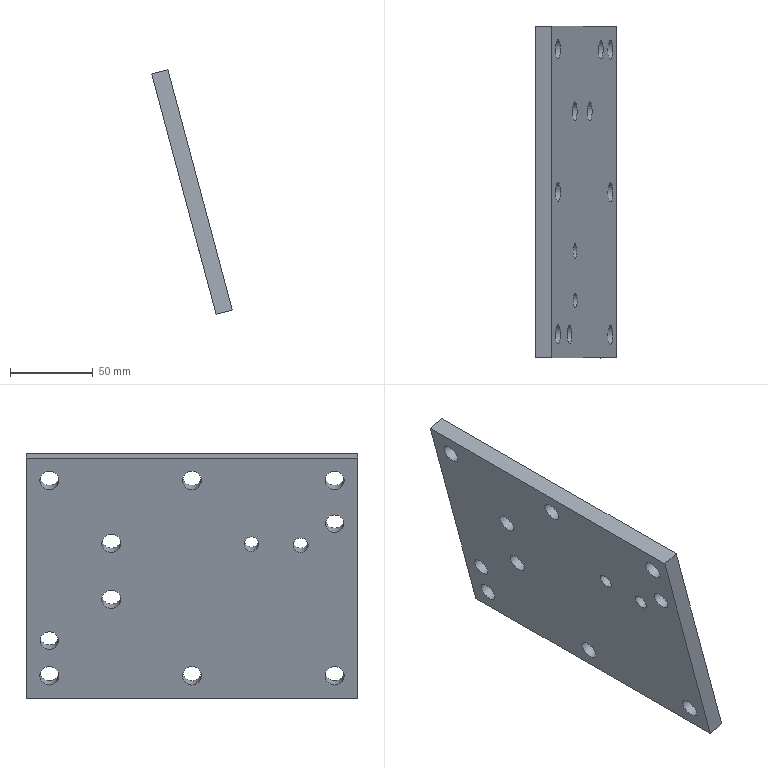Part | NX | features solid 2 | 1 solid | 18 faces | box 48.482 x 200 x 147.477 mm | volume 288505 mm3 | cylinder 12 | plane 6 | commonest cylinder face diameters 11.507 x8 9.007 x2 11 x2
STEP:
#1=CARTESIAN_POINT('',(922.389,65.937,-48.234));
#2=VERTEX_POINT('',#1);
#3=CARTESIAN_POINT('',(920.965,65.937,-42.921));
#4=DIRECTION('',(0.9659,-0.000000134,0.2588));
#5=DIRECTION('',(0.2588,0.,-0.9659));
#6=AXIS2_PLACEMENT_3D('',#3,#4,#5);
#7=CIRCLE('',#6,5.5);
#8=EDGE_CURVE('',#2,#2,#7,.F.);
#9=ORIENTED_EDGE('',*,*,#8,.F.);
#10=EDGE_LOOP('',(#9));
#11=FACE_BOUND('',#10,.T.);
#12=CARTESIAN_POINT('',(896.573,-20.063,48.114));
#13=VERTEX_POINT('',#12);
#14=CARTESIAN_POINT('',(895.084,-20.063,53.671));
#15=DIRECTION('',(0.9659,-0.000000134,0.2588));
#16=DIRECTION('',(0.2588,0.,-0.9659));
#17=AXIS2_PLACEMENT_3D('',#14,#15,#16);
#18=CIRCLE('',#17,5.753);
#19=EDGE_CURVE('',#13,#13,#18,.F.);
#20=ORIENTED_EDGE('',*,*,#19,.F.);
#21=EDGE_LOOP('',(#20));
#22=FACE_BOUND('',#21,.T.);
#23=CARTESIAN_POINT('',(928.149,-20.063,-69.729));
#24=VERTEX_POINT('',#23);
#25=CARTESIAN_POINT('',(926.659,-20.063,-64.172));
#26=DIRECTION('',(0.9659,-0.000000134,0.2588));
#27=DIRECTION('',(0.2588,0.,-0.9659));
#28=AXIS2_PLACEMENT_3D('',#25,#26,#27);
#29=CIRCLE('',#28,5.753);
#30=EDGE_CURVE('',#24,#24,#29,.T.);
#31=ORIENTED_EDGE('',*,*,#30,.T.);
#32=EDGE_LOOP('',(#31));
#33=FACE_BOUND('',#32,.T.);
#34=CARTESIAN_POINT('',(928.149,65.937,-69.729));
#35=VERTEX_POINT('',#34);
#36=CARTESIAN_POINT('',(926.659,65.937,-64.172));
#37=DIRECTION('',(0.9659,-0.000000134,0.2588));
#38=DIRECTION('',(0.2588,0.,-0.9659));
#39=AXIS2_PLACEMENT_3D('',#36,#37,#38);
#40=CIRCLE('',#39,5.753);
#41=EDGE_CURVE('',#35,#35,#40,.T.);
#42=ORIENTED_EDGE('',*,*,#41,.T.);
#43=EDGE_LOOP('',(#42));
#44=FACE_BOUND('',#43,.T.);
#45=CARTESIAN_POINT('',(891.46,-120.063,67.194));
#46=VERTEX_POINT('',#45);
#47=CARTESIAN_POINT('',(930.283,-120.063,-77.695));
#48=VERTEX_POINT('',#47);
#49=CARTESIAN_POINT('',(1072.537,-120.063,-608.595));
#50=DIRECTION('',(0.2588,0.000000499,-0.9659));
#51=VECTOR('',#50,1000.);
#52=LINE('',#49,#51);
#53=EDGE_CURVE('',#46,#48,#52,.T.);
#54=ORIENTED_EDGE('',*,*,#53,.F.);
#55=CARTESIAN_POINT('',(891.46,79.937,67.194));
#56=VERTEX_POINT('',#55);
#57=CARTESIAN_POINT('',(891.46,4.19,67.194));
#58=DIRECTION('',(0.,-1.,-0.000000517));
#59=VECTOR('',#58,1000.);
#60=LINE('',#57,#59);
#61=EDGE_CURVE('',#56,#46,#60,.T.);
#62=ORIENTED_EDGE('',*,*,#61,.F.);
#63=CARTESIAN_POINT('',(930.283,79.937,-77.695));
#64=VERTEX_POINT('',#63);
#65=CARTESIAN_POINT('',(925.107,79.937,-58.376));
#66=DIRECTION('',(-0.2588,-0.000000499,0.9659));
#67=VECTOR('',#66,1000.);
#68=LINE('',#65,#67);
#69=EDGE_CURVE('',#64,#56,#68,.T.);
#70=ORIENTED_EDGE('',*,*,#69,.F.);
#71=CARTESIAN_POINT('',(930.283,-100.063,-77.695));
#72=DIRECTION('',(0.,1.,0.000000517));
#73=VECTOR('',#72,1000.);
#74=LINE('',#71,#73);
#75=EDGE_CURVE('',#48,#64,#74,.T.);
#76=ORIENTED_EDGE('',*,*,#75,.F.);
#77=EDGE_LOOP('',(#54,#62,#70,#76));
#78=FACE_BOUND('',#77,.T.);
#79=CARTESIAN_POINT('',(915.774,28.571,-23.546));
#80=VERTEX_POINT('',#79);
#81=CARTESIAN_POINT('',(914.285,28.571,-17.988));
#82=DIRECTION('',(0.9659,-0.000000134,0.2588));
#83=DIRECTION('',(0.2588,0.,-0.9659));
#84=AXIS2_PLACEMENT_3D('',#81,#82,#83);
#85=CIRCLE('',#84,5.753);
#86=EDGE_CURVE('',#80,#80,#85,.T.);
#87=ORIENTED_EDGE('',*,*,#86,.T.);
#88=EDGE_LOOP('',(#87));
#89=FACE_BOUND('',#88,.T.);
#90=CARTESIAN_POINT('',(906.716,-85.584,10.259));
#91=VERTEX_POINT('',#90);
#92=CARTESIAN_POINT('',(905.55,-85.584,14.61));
#93=DIRECTION('',(0.9659,-0.000000134,0.2588));
#94=DIRECTION('',(0.2588,0.,-0.9659));
#95=AXIS2_PLACEMENT_3D('',#92,#93,#94);
#96=CIRCLE('',#95,4.503);
#97=EDGE_CURVE('',#91,#91,#96,.T.);
#98=ORIENTED_EDGE('',*,*,#97,.T.);
#99=EDGE_LOOP('',(#98));
#100=FACE_BOUND('',#99,.T.);
#101=CARTESIAN_POINT('',(906.538,-55.901,10.924));
#102=VERTEX_POINT('',#101);
#103=CARTESIAN_POINT('',(905.372,-55.901,15.274));
#104=DIRECTION('',(0.9659,-0.000000134,0.2588));
#105=DIRECTION('',(0.2588,0.,-0.9659));
#106=AXIS2_PLACEMENT_3D('',#103,#104,#105);
#107=CIRCLE('',#106,4.503);
#108=EDGE_CURVE('',#102,#102,#107,.T.);
#109=ORIENTED_EDGE('',*,*,#108,.T.);
#110=EDGE_LOOP('',(#109));
#111=FACE_BOUND('',#110,.T.);
#112=CARTESIAN_POINT('',(906.735,28.571,10.189));
#113=VERTEX_POINT('',#112);
#114=CARTESIAN_POINT('',(905.245,28.571,15.746));
#115=DIRECTION('',(0.9659,-0.000000134,0.2588));
#116=DIRECTION('',(0.2588,0.,-0.9659));
#117=AXIS2_PLACEMENT_3D('',#114,#115,#116);
#118=CIRCLE('',#117,5.753);
#119=EDGE_CURVE('',#113,#113,#118,.F.);
#120=ORIENTED_EDGE('',*,*,#119,.F.);
#121=EDGE_LOOP('',(#120));
#122=FACE_BOUND('',#121,.T.);
#123=CARTESIAN_POINT('',(896.573,-106.063,48.114));
#124=VERTEX_POINT('',#123);
#125=CARTESIAN_POINT('',(895.084,-106.063,53.671));
#126=DIRECTION('',(0.9659,-0.000000134,0.2588));
#127=DIRECTION('',(0.2588,0.,-0.9659));
#128=AXIS2_PLACEMENT_3D('',#125,#126,#127);
#129=CIRCLE('',#128,5.753);
#130=EDGE_CURVE('',#124,#124,#129,.T.);
#131=ORIENTED_EDGE('',*,*,#130,.T.);
#132=EDGE_LOOP('',(#131));
#133=FACE_BOUND('',#132,.T.);
#134=CARTESIAN_POINT('',(896.573,65.937,48.114));
#135=VERTEX_POINT('',#134);
#136=CARTESIAN_POINT('',(895.084,65.937,53.671));
#137=DIRECTION('',(0.9659,-0.000000134,0.2588));
#138=DIRECTION('',(0.2588,0.,-0.9659));
#139=AXIS2_PLACEMENT_3D('',#136,#137,#138);
#140=CIRCLE('',#139,5.753);
#141=EDGE_CURVE('',#135,#135,#140,.T.);
#142=ORIENTED_EDGE('',*,*,#141,.T.);
#143=EDGE_LOOP('',(#142));
#144=FACE_BOUND('',#143,.T.);
#145=CARTESIAN_POINT('',(928.149,-106.063,-69.729));
#146=VERTEX_POINT('',#145);
#147=CARTESIAN_POINT('',(926.659,-106.063,-64.172));
#148=DIRECTION('',(0.9659,-0.000000134,0.2588));
#149=DIRECTION('',(0.2588,0.,-0.9659));
#150=AXIS2_PLACEMENT_3D('',#147,#148,#149);
#151=CIRCLE('',#150,5.753);
#152=EDGE_CURVE('',#146,#146,#151,.F.);
#153=ORIENTED_EDGE('',*,*,#152,.F.);
#154=EDGE_LOOP('',(#153));
#155=FACE_BOUND('',#154,.T.);
#156=CARTESIAN_POINT('',(903.495,-106.063,22.279));
#157=VERTEX_POINT('',#156);
#158=CARTESIAN_POINT('',(902.072,-106.063,27.591));
#159=DIRECTION('',(0.9659,-0.000000134,0.2588));
#160=DIRECTION('',(0.2588,0.,-0.9659));
#161=AXIS2_PLACEMENT_3D('',#158,#159,#160);
#162=CIRCLE('',#161,5.5);
#163=EDGE_CURVE('',#157,#157,#162,.F.);
#164=ORIENTED_EDGE('',*,*,#163,.F.);
#165=EDGE_LOOP('',(#164));
#166=FACE_BOUND('',#165,.T.);
#167=CARTESIAN_POINT('',(1072.537,4.191,-608.595));
#168=DIRECTION('',(0.9659,-0.000000134,0.2588));
#169=DIRECTION('',(-0.2588,0.,0.9659));
#170=AXIS2_PLACEMENT_3D('',#167,#168,#169);
#171=PLANE('',#170);
#172=ADVANCED_FACE('',(#11,#22,#33,#44,#78,#89,#100,#111,#122,#133,#144,#155,#166),#171,.F.);
#173=CARTESIAN_POINT('',(932.048,65.937,-45.646));
#174=VERTEX_POINT('',#173);
#175=CARTESIAN_POINT('',(930.625,65.937,-40.333));
#176=DIRECTION('',(0.9659,-0.000000134,0.2588));
#177=DIRECTION('',(0.2588,0.,-0.9659));
#178=AXIS2_PLACEMENT_3D('',#175,#176,#177);
#179=CIRCLE('',#178,5.5);
#180=EDGE_CURVE('',#174,#174,#179,.F.);
#181=ORIENTED_EDGE('',*,*,#180,.T.);
#182=EDGE_LOOP('',(#181));
#183=FACE_BOUND('',#182,.T.);
#184=CARTESIAN_POINT('',(906.232,-20.063,50.702));
#185=VERTEX_POINT('',#184);
#186=CARTESIAN_POINT('',(904.743,-20.063,56.259));
#187=DIRECTION('',(0.9659,-0.000000134,0.2588));
#188=DIRECTION('',(0.2588,0.,-0.9659));
#189=AXIS2_PLACEMENT_3D('',#186,#187,#188);
#190=CIRCLE('',#189,5.753);
#191=EDGE_CURVE('',#185,#185,#190,.F.);
#192=ORIENTED_EDGE('',*,*,#191,.T.);
#193=EDGE_LOOP('',(#192));
#194=FACE_BOUND('',#193,.T.);
#195=CARTESIAN_POINT('',(937.808,-20.063,-67.141));
#196=VERTEX_POINT('',#195);
#197=CARTESIAN_POINT('',(936.319,-20.063,-61.584));
#198=DIRECTION('',(0.9659,-0.000000134,0.2588));
#199=DIRECTION('',(0.2588,0.,-0.9659));
#200=AXIS2_PLACEMENT_3D('',#197,#198,#199);
#201=CIRCLE('',#200,5.753);
#202=EDGE_CURVE('',#196,#196,#201,.T.);
#203=ORIENTED_EDGE('',*,*,#202,.F.);
#204=EDGE_LOOP('',(#203));
#205=FACE_BOUND('',#204,.T.);
#206=CARTESIAN_POINT('',(937.808,65.937,-67.141));
#207=VERTEX_POINT('',#206);
#208=CARTESIAN_POINT('',(936.319,65.937,-61.584));
#209=DIRECTION('',(0.9659,-0.000000134,0.2588));
#210=DIRECTION('',(0.2588,0.,-0.9659));
#211=AXIS2_PLACEMENT_3D('',#208,#209,#210);
#212=CIRCLE('',#211,5.753);
#213=EDGE_CURVE('',#207,#207,#212,.T.);
#214=ORIENTED_EDGE('',*,*,#213,.F.);
#215=EDGE_LOOP('',(#214));
#216=FACE_BOUND('',#215,.T.);
#217=CARTESIAN_POINT('',(901.119,-120.063,69.782));
#218=VERTEX_POINT('',#217);
#219=CARTESIAN_POINT('',(939.942,-120.063,-75.107));
#220=VERTEX_POINT('',#219);
#221=CARTESIAN_POINT('',(1082.196,-120.063,-606.006));
#222=DIRECTION('',(0.2588,0.000000499,-0.9659));
#223=VECTOR('',#222,1000.);
#224=LINE('',#221,#223);
#225=EDGE_CURVE('',#218,#220,#224,.T.);
#226=ORIENTED_EDGE('',*,*,#225,.T.);
#227=CARTESIAN_POINT('',(939.942,79.937,-75.107));
#228=VERTEX_POINT('',#227);
#229=CARTESIAN_POINT('',(939.942,-100.063,-75.107));
#230=DIRECTION('',(0.,1.,0.000000517));
#231=VECTOR('',#230,1000.);
#232=LINE('',#229,#231);
#233=EDGE_CURVE('',#220,#228,#232,.T.);
#234=ORIENTED_EDGE('',*,*,#233,.T.);
#235=CARTESIAN_POINT('',(901.119,79.937,69.782));
#236=VERTEX_POINT('',#235);
#237=CARTESIAN_POINT('',(934.766,79.937,-55.788));
#238=DIRECTION('',(-0.2588,-0.000000499,0.9659));
#239=VECTOR('',#238,1000.);
#240=LINE('',#237,#239);
#241=EDGE_CURVE('',#228,#236,#240,.T.);
#242=ORIENTED_EDGE('',*,*,#241,.T.);
#243=CARTESIAN_POINT('',(901.119,4.19,69.782));
#244=DIRECTION('',(0.,-1.,-0.000000517));
#245=VECTOR('',#244,1000.);
#246=LINE('',#243,#245);
#247=EDGE_CURVE('',#236,#218,#246,.T.);
#248=ORIENTED_EDGE('',*,*,#247,.T.);
#249=EDGE_LOOP('',(#226,#234,#242,#248));
#250=FACE_BOUND('',#249,.T.);
#251=CARTESIAN_POINT('',(925.433,28.571,-20.957));
#252=VERTEX_POINT('',#251);
#253=CARTESIAN_POINT('',(923.944,28.571,-15.4));
#254=DIRECTION('',(0.9659,-0.000000134,0.2588));
#255=DIRECTION('',(0.2588,0.,-0.9659));
#256=AXIS2_PLACEMENT_3D('',#253,#254,#255);
#257=CIRCLE('',#256,5.753);
#258=EDGE_CURVE('',#252,#252,#257,.T.);
#259=ORIENTED_EDGE('',*,*,#258,.F.);
#260=EDGE_LOOP('',(#259));
#261=FACE_BOUND('',#260,.T.);
#262=CARTESIAN_POINT('',(916.375,-85.584,12.848));
#263=VERTEX_POINT('',#262);
#264=CARTESIAN_POINT('',(915.209,-85.584,17.198));
#265=DIRECTION('',(0.9659,-0.000000134,0.2588));
#266=DIRECTION('',(0.2588,0.,-0.9659));
#267=AXIS2_PLACEMENT_3D('',#264,#265,#266);
#268=CIRCLE('',#267,4.503);
#269=EDGE_CURVE('',#263,#263,#268,.T.);
#270=ORIENTED_EDGE('',*,*,#269,.F.);
#271=EDGE_LOOP('',(#270));
#272=FACE_BOUND('',#271,.T.);
#273=CARTESIAN_POINT('',(916.197,-55.901,13.512));
#274=VERTEX_POINT('',#273);
#275=CARTESIAN_POINT('',(915.031,-55.901,17.862));
#276=DIRECTION('',(0.9659,-0.000000134,0.2588));
#277=DIRECTION('',(0.2588,0.,-0.9659));
#278=AXIS2_PLACEMENT_3D('',#275,#276,#277);
#279=CIRCLE('',#278,4.503);
#280=EDGE_CURVE('',#274,#274,#279,.T.);
#281=ORIENTED_EDGE('',*,*,#280,.F.);
#282=EDGE_LOOP('',(#281));
#283=FACE_BOUND('',#282,.T.);
#284=CARTESIAN_POINT('',(916.394,28.571,12.777));
#285=VERTEX_POINT('',#284);
#286=CARTESIAN_POINT('',(914.905,28.571,18.335));
#287=DIRECTION('',(0.9659,-0.000000134,0.2588));
#288=DIRECTION('',(0.2588,0.,-0.9659));
#289=AXIS2_PLACEMENT_3D('',#286,#287,#288);
#290=CIRCLE('',#289,5.753);
#291=EDGE_CURVE('',#285,#285,#290,.F.);
#292=ORIENTED_EDGE('',*,*,#291,.T.);
#293=EDGE_LOOP('',(#292));
#294=FACE_BOUND('',#293,.T.);
#295=CARTESIAN_POINT('',(906.232,-106.063,50.702));
#296=VERTEX_POINT('',#295);
#297=CARTESIAN_POINT('',(904.743,-106.063,56.259));
#298=DIRECTION('',(0.9659,-0.000000134,0.2588));
#299=DIRECTION('',(0.2588,0.,-0.9659));
#300=AXIS2_PLACEMENT_3D('',#297,#298,#299);
#301=CIRCLE('',#300,5.753);
#302=EDGE_CURVE('',#296,#296,#301,.T.);
#303=ORIENTED_EDGE('',*,*,#302,.F.);
#304=EDGE_LOOP('',(#303));
#305=FACE_BOUND('',#304,.T.);
#306=CARTESIAN_POINT('',(906.232,65.937,50.702));
#307=VERTEX_POINT('',#306);
#308=CARTESIAN_POINT('',(904.743,65.937,56.259));
#309=DIRECTION('',(0.9659,-0.000000134,0.2588));
#310=DIRECTION('',(0.2588,0.,-0.9659));
#311=AXIS2_PLACEMENT_3D('',#308,#309,#310);
#312=CIRCLE('',#311,5.753);
#313=EDGE_CURVE('',#307,#307,#312,.T.);
#314=ORIENTED_EDGE('',*,*,#313,.F.);
#315=EDGE_LOOP('',(#314));
#316=FACE_BOUND('',#315,.T.);
#317=CARTESIAN_POINT('',(937.808,-106.063,-67.141));
#318=VERTEX_POINT('',#317);
#319=CARTESIAN_POINT('',(936.319,-106.063,-61.584));
#320=DIRECTION('',(0.9659,-0.000000134,0.2588));
#321=DIRECTION('',(0.2588,0.,-0.9659));
#322=AXIS2_PLACEMENT_3D('',#319,#320,#321);
#323=CIRCLE('',#322,5.753);
#324=EDGE_CURVE('',#318,#318,#323,.F.);
#325=ORIENTED_EDGE('',*,*,#324,.T.);
#326=EDGE_LOOP('',(#325));
#327=FACE_BOUND('',#326,.T.);
#328=CARTESIAN_POINT('',(913.154,-106.063,24.867));
#329=VERTEX_POINT('',#328);
#330=CARTESIAN_POINT('',(911.731,-106.063,30.179));
#331=DIRECTION('',(0.9659,-0.000000134,0.2588));
#332=DIRECTION('',(0.2588,0.,-0.9659));
#333=AXIS2_PLACEMENT_3D('',#330,#331,#332);
#334=CIRCLE('',#333,5.5);
#335=EDGE_CURVE('',#329,#329,#334,.F.);
#336=ORIENTED_EDGE('',*,*,#335,.T.);
#337=EDGE_LOOP('',(#336));
#338=FACE_BOUND('',#337,.T.);
#339=CARTESIAN_POINT('',(1082.196,4.191,-606.006));
#340=DIRECTION('',(0.9659,-0.000000134,0.2588));
#341=DIRECTION('',(-0.2588,0.,0.9659));
#342=AXIS2_PLACEMENT_3D('',#339,#340,#341);
#343=PLANE('',#342);
#344=ADVANCED_FACE('',(#183,#194,#205,#216,#250,#261,#272,#283,#294,#305,#316,#327,#338),#343,.T.);
#345=ORIENTED_EDGE('',*,*,#225,.F.);
#346=CARTESIAN_POINT('',(881.801,-120.063,64.606));
#347=DIRECTION('',(0.9659,-0.000000134,0.2588));
#348=VECTOR('',#347,1000.);
#349=LINE('',#346,#348);
#350=EDGE_CURVE('',#46,#218,#349,.T.);
#351=ORIENTED_EDGE('',*,*,#350,.F.);
#352=ORIENTED_EDGE('',*,*,#53,.T.);
#353=CARTESIAN_POINT('',(920.624,-120.063,-80.283));
#354=DIRECTION('',(0.9659,-0.000000134,0.2588));
#355=VECTOR('',#354,1000.);
#356=LINE('',#353,#355);
#357=EDGE_CURVE('',#48,#220,#356,.T.);
#358=ORIENTED_EDGE('',*,*,#357,.T.);
#359=EDGE_LOOP('',(#345,#351,#352,#358));
#360=FACE_BOUND('',#359,.T.);
#361=CARTESIAN_POINT('',(874.036,-120.063,93.584));
#362=DIRECTION('',(0.,-1.,-0.000000517));
#363=DIRECTION('',(0.,-0.000000517,1.));
#364=AXIS2_PLACEMENT_3D('',#361,#362,#363);
#365=PLANE('',#364);
#366=ADVANCED_FACE('',(#360),#365,.T.);
#367=ORIENTED_EDGE('',*,*,#233,.F.);
#368=ORIENTED_EDGE('',*,*,#357,.F.);
#369=ORIENTED_EDGE('',*,*,#75,.T.);
#370=CARTESIAN_POINT('',(920.624,79.937,-80.283));
#371=DIRECTION('',(0.9659,-0.000000134,0.2588));
#372=VECTOR('',#371,1000.);
#373=LINE('',#370,#372);
#374=EDGE_CURVE('',#64,#228,#373,.T.);
#375=ORIENTED_EDGE('',*,*,#374,.T.);
#376=EDGE_LOOP('',(#367,#368,#369,#375));
#377=FACE_BOUND('',#376,.T.);
#378=CARTESIAN_POINT('',(920.624,-100.063,-80.283));
#379=DIRECTION('',(0.2588,0.000000499,-0.9659));
#380=DIRECTION('',(0.9659,0.,0.2588));
#381=AXIS2_PLACEMENT_3D('',#378,#379,#380);
#382=PLANE('',#381);
#383=ADVANCED_FACE('',(#377),#382,.T.);
#384=ORIENTED_EDGE('',*,*,#241,.F.);
#385=ORIENTED_EDGE('',*,*,#374,.F.);
#386=ORIENTED_EDGE('',*,*,#69,.T.);
#387=CARTESIAN_POINT('',(881.801,79.937,64.606));
#388=DIRECTION('',(0.9659,-0.000000134,0.2588));
#389=VECTOR('',#388,1000.);
#390=LINE('',#387,#389);
#391=EDGE_CURVE('',#56,#236,#390,.T.);
#392=ORIENTED_EDGE('',*,*,#391,.T.);
#393=EDGE_LOOP('',(#384,#385,#386,#392));
#394=FACE_BOUND('',#393,.T.);
#395=CARTESIAN_POINT('',(915.447,79.937,-60.964));
#396=DIRECTION('',(0.,1.,0.000000517));
#397=DIRECTION('',(0.,0.000000517,-1.));
#398=AXIS2_PLACEMENT_3D('',#395,#396,#397);
#399=PLANE('',#398);
#400=ADVANCED_FACE('',(#394),#399,.T.);
#401=ORIENTED_EDGE('',*,*,#247,.F.);
#402=ORIENTED_EDGE('',*,*,#391,.F.);
#403=ORIENTED_EDGE('',*,*,#61,.T.);
#404=ORIENTED_EDGE('',*,*,#350,.T.);
#405=EDGE_LOOP('',(#401,#402,#403,#404));
#406=FACE_BOUND('',#405,.T.);
#407=CARTESIAN_POINT('',(881.801,79.937,64.606));
#408=DIRECTION('',(-0.2588,-0.000000499,0.9659));
#409=DIRECTION('',(-0.9659,0.,-0.2588));
#410=AXIS2_PLACEMENT_3D('',#407,#408,#409);
#411=PLANE('',#410);
#412=ADVANCED_FACE('',(#406),#411,.T.);
#413=ORIENTED_EDGE('',*,*,#258,.T.);
#414=EDGE_LOOP('',(#413));
#415=FACE_BOUND('',#414,.T.);
#416=ORIENTED_EDGE('',*,*,#86,.F.);
#417=EDGE_LOOP('',(#416));
#418=FACE_BOUND('',#417,.T.);
#419=CARTESIAN_POINT('',(58.708,28.571,-247.239));
#420=DIRECTION('',(0.9659,-0.000000134,0.2588));
#421=DIRECTION('',(0.2588,0.,-0.9659));
#422=AXIS2_PLACEMENT_3D('',#419,#420,#421);
#423=CYLINDRICAL_SURFACE('',#422,5.753);
#424=ADVANCED_FACE('',(#415,#418),#423,.F.);
#425=ORIENTED_EDGE('',*,*,#269,.T.);
#426=EDGE_LOOP('',(#425));
#427=FACE_BOUND('',#426,.T.);
#428=ORIENTED_EDGE('',*,*,#97,.F.);
#429=EDGE_LOOP('',(#428));
#430=FACE_BOUND('',#429,.T.);
#431=CARTESIAN_POINT('',(49.973,-85.584,-214.642));
#432=DIRECTION('',(0.9659,-0.000000134,0.2588));
#433=DIRECTION('',(0.2588,0.,-0.9659));
#434=AXIS2_PLACEMENT_3D('',#431,#432,#433);
#435=CYLINDRICAL_SURFACE('',#434,4.503);
#436=ADVANCED_FACE('',(#427,#430),#435,.F.);
#437=ORIENTED_EDGE('',*,*,#280,.T.);
#438=EDGE_LOOP('',(#437));
#439=FACE_BOUND('',#438,.T.);
#440=ORIENTED_EDGE('',*,*,#108,.F.);
#441=EDGE_LOOP('',(#440));
#442=FACE_BOUND('',#441,.T.);
#443=CARTESIAN_POINT('',(49.795,-55.901,-213.978));
#444=DIRECTION('',(0.9659,-0.000000134,0.2588));
#445=DIRECTION('',(0.2588,0.,-0.9659));
#446=AXIS2_PLACEMENT_3D('',#443,#444,#445);
#447=CYLINDRICAL_SURFACE('',#446,4.503);
#448=ADVANCED_FACE('',(#439,#442),#447,.F.);
#449=ORIENTED_EDGE('',*,*,#291,.F.);
#450=EDGE_LOOP('',(#449));
#451=FACE_BOUND('',#450,.T.);
#452=ORIENTED_EDGE('',*,*,#119,.T.);
#453=EDGE_LOOP('',(#452));
#454=FACE_BOUND('',#453,.T.);
#455=CARTESIAN_POINT('',(49.669,28.571,-213.505));
#456=DIRECTION('',(0.9659,-0.000000134,0.2588));
#457=DIRECTION('',(0.2588,0.,-0.9659));
#458=AXIS2_PLACEMENT_3D('',#455,#456,#457);
#459=CYLINDRICAL_SURFACE('',#458,5.753);
#460=ADVANCED_FACE('',(#451,#454),#459,.F.);
#461=ORIENTED_EDGE('',*,*,#213,.T.);
#462=EDGE_LOOP('',(#461));
#463=FACE_BOUND('',#462,.T.);
#464=ORIENTED_EDGE('',*,*,#41,.F.);
#465=EDGE_LOOP('',(#464));
#466=FACE_BOUND('',#465,.T.);
#467=CARTESIAN_POINT('',(115.282,65.937,-281.58));
#468=DIRECTION('',(0.9659,-0.000000134,0.2588));
#469=DIRECTION('',(0.2588,0.,-0.9659));
#470=AXIS2_PLACEMENT_3D('',#467,#468,#469);
#471=CYLINDRICAL_SURFACE('',#470,5.753);
#472=ADVANCED_FACE('',(#463,#466),#471,.F.);
#473=ORIENTED_EDGE('',*,*,#202,.T.);
#474=EDGE_LOOP('',(#473));
#475=FACE_BOUND('',#474,.T.);
#476=ORIENTED_EDGE('',*,*,#30,.F.);
#477=EDGE_LOOP('',(#476));
#478=FACE_BOUND('',#477,.T.);
#479=CARTESIAN_POINT('',(115.282,-20.063,-281.58));
#480=DIRECTION('',(0.9659,-0.000000134,0.2588));
#481=DIRECTION('',(0.2588,0.,-0.9659));
#482=AXIS2_PLACEMENT_3D('',#479,#480,#481);
#483=CYLINDRICAL_SURFACE('',#482,5.753);
#484=ADVANCED_FACE('',(#475,#478),#483,.F.);
#485=ORIENTED_EDGE('',*,*,#191,.F.);
#486=EDGE_LOOP('',(#485));
#487=FACE_BOUND('',#486,.T.);
#488=ORIENTED_EDGE('',*,*,#19,.T.);
#489=EDGE_LOOP('',(#488));
#490=FACE_BOUND('',#489,.T.);
#491=CARTESIAN_POINT('',(83.706,-20.063,-163.737));
#492=DIRECTION('',(0.9659,-0.000000134,0.2588));
#493=DIRECTION('',(0.2588,0.,-0.9659));
#494=AXIS2_PLACEMENT_3D('',#491,#492,#493);
#495=CYLINDRICAL_SURFACE('',#494,5.753);
#496=ADVANCED_FACE('',(#487,#490),#495,.F.);
#497=ORIENTED_EDGE('',*,*,#302,.T.);
#498=EDGE_LOOP('',(#497));
#499=FACE_BOUND('',#498,.T.);
#500=ORIENTED_EDGE('',*,*,#130,.F.);
#501=EDGE_LOOP('',(#500));
#502=FACE_BOUND('',#501,.T.);
#503=CARTESIAN_POINT('',(83.706,-106.063,-163.737));
#504=DIRECTION('',(0.9659,-0.000000134,0.2588));
#505=DIRECTION('',(0.2588,0.,-0.9659));
#506=AXIS2_PLACEMENT_3D('',#503,#504,#505);
#507=CYLINDRICAL_SURFACE('',#506,5.753);
#508=ADVANCED_FACE('',(#499,#502),#507,.F.);
#509=ORIENTED_EDGE('',*,*,#313,.T.);
#510=EDGE_LOOP('',(#509));
#511=FACE_BOUND('',#510,.T.);
#512=ORIENTED_EDGE('',*,*,#141,.F.);
#513=EDGE_LOOP('',(#512));
#514=FACE_BOUND('',#513,.T.);
#515=CARTESIAN_POINT('',(83.706,65.937,-163.737));
#516=DIRECTION('',(0.9659,-0.000000134,0.2588));
#517=DIRECTION('',(0.2588,0.,-0.9659));
#518=AXIS2_PLACEMENT_3D('',#515,#516,#517);
#519=CYLINDRICAL_SURFACE('',#518,5.753);
#520=ADVANCED_FACE('',(#511,#514),#519,.F.);
#521=ORIENTED_EDGE('',*,*,#324,.F.);
#522=EDGE_LOOP('',(#521));
#523=FACE_BOUND('',#522,.T.);
#524=ORIENTED_EDGE('',*,*,#152,.T.);
#525=EDGE_LOOP('',(#524));
#526=FACE_BOUND('',#525,.T.);
#527=CARTESIAN_POINT('',(115.282,-106.063,-281.58));
#528=DIRECTION('',(0.9659,-0.000000134,0.2588));
#529=DIRECTION('',(0.2588,0.,-0.9659));
#530=AXIS2_PLACEMENT_3D('',#527,#528,#529);
#531=CYLINDRICAL_SURFACE('',#530,5.753);
#532=ADVANCED_FACE('',(#523,#526),#531,.F.);
#533=ORIENTED_EDGE('',*,*,#180,.F.);
#534=EDGE_LOOP('',(#533));
#535=FACE_BOUND('',#534,.T.);
#536=ORIENTED_EDGE('',*,*,#8,.T.);
#537=EDGE_LOOP('',(#536));
#538=FACE_BOUND('',#537,.T.);
#539=CARTESIAN_POINT('',(1693.706,65.937,164.134));
#540=DIRECTION('',(-0.9659,0.000000134,-0.2588));
#541=DIRECTION('',(-0.2588,0.,0.9659));
#542=AXIS2_PLACEMENT_3D('',#539,#540,#541);
#543=CYLINDRICAL_SURFACE('',#542,5.5);
#544=ADVANCED_FACE('',(#535,#538),#543,.F.);
#545=ORIENTED_EDGE('',*,*,#335,.F.);
#546=EDGE_LOOP('',(#545));
#547=FACE_BOUND('',#546,.T.);
#548=ORIENTED_EDGE('',*,*,#163,.T.);
#549=EDGE_LOOP('',(#548));
#550=FACE_BOUND('',#549,.T.);
#551=CARTESIAN_POINT('',(1674.812,-106.063,234.646));
#552=DIRECTION('',(-0.9659,0.000000134,-0.2588));
#553=DIRECTION('',(-0.2588,0.,0.9659));
#554=AXIS2_PLACEMENT_3D('',#551,#552,#553);
#555=CYLINDRICAL_SURFACE('',#554,5.5);
#556=ADVANCED_FACE('',(#547,#550),#555,.F.);
#557=CLOSED_SHELL('',(#172,#344,#366,#383,#400,#412,#424,#436,#448,#460,#472,#484,#496,#508,#520,#532,#544,#556));
#558=MANIFOLD_SOLID_BREP('',#557);
#559=(LENGTH_UNIT()NAMED_UNIT(*)SI_UNIT(.MILLI.,.METRE.));
#560=UNCERTAINTY_MEASURE_WITH_UNIT(LENGTH_MEASURE(0.00001),#559,'','');
#561=(NAMED_UNIT(*)PLANE_ANGLE_UNIT()SI_UNIT($,.RADIAN.));
#562=(NAMED_UNIT(*)SI_UNIT($,.STERADIAN.)SOLID_ANGLE_UNIT());
#563=(GEOMETRIC_REPRESENTATION_CONTEXT(3)GLOBAL_UNCERTAINTY_ASSIGNED_CONTEXT((#560))GLOBAL_UNIT_ASSIGNED_CONTEXT((#559,#561,#562))REPRESENTATION_CONTEXT('',''));
#564=ADVANCED_BREP_SHAPE_REPRESENTATION('',(#558),#563);